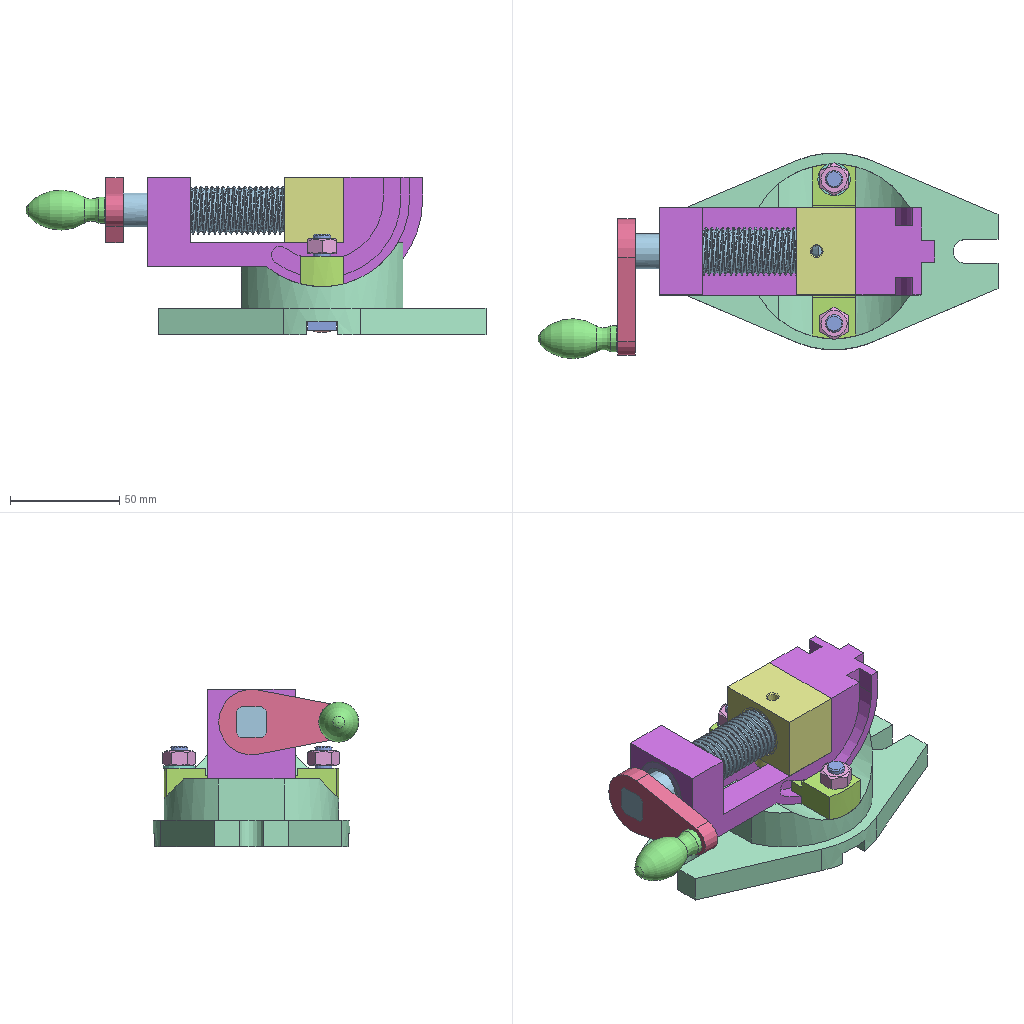Assembly | NX | 12 different items | 15 placed | box 210 x 94 x 72 mm
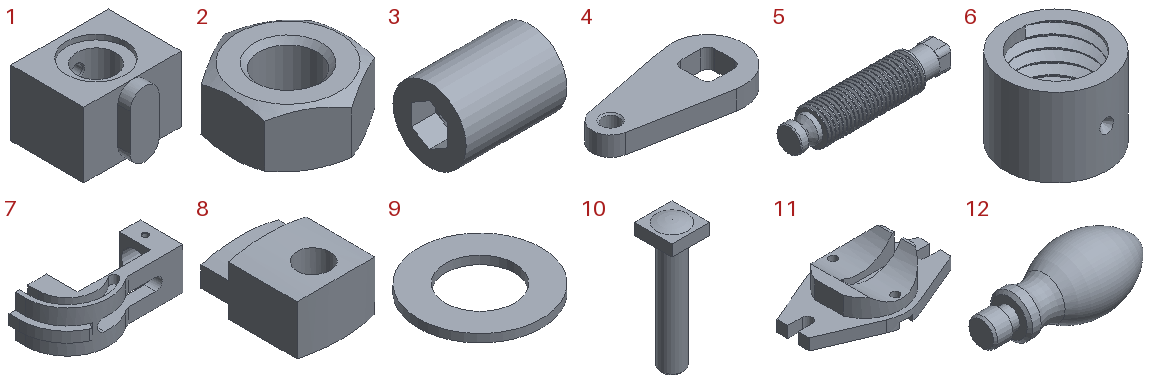Parts list (item | quantity | size | volume | features):
1 | x1 | 40 x 35 x 27 mm | 30203 mm3 | features DATUM_CSYS 6, SKETCH 5, EXTRUDE 4, BLEND 1, HOLE PACKAGE 1, SIMPLE HOLE 1, SYMBOLIC_THREAD 1
2 | x2 | 12.99 x 15 x 6.8 mm | 720.374 mm3 | features DATUM_CSYS 3, EXTRACT_DATUM_AXIS 2, EXTRACT_STRING 2, SKETCH 2, SWP104 2, EXTRUDE 1, HOLE PACKAGE 1, Instance Feature 1, Mirror Feature 1, SIMPLE HOLE 1, SYMBOLIC_THREAD 1
3 | x1 | 10 x 6 x 6 mm | 232.466 mm3 | features DATUM_CSYS 4, SKETCH 3, SWP104 2, EXTRUDE 1
4 | x1 | 62.5 x 30 x 8 mm | 9056 mm3 | features DATUM_CSYS 2, BLEND 1, EXTRUDE 1, HOLE PACKAGE 1, SIMPLE HOLE 1, SKETCH 1, SYMBOLIC_THREAD 1
5 | x1 | 97 x 22 x 22 mm | 27588 mm3 | features DATUM_CSYS 3, SKETCH 2, BLEND 1, CHAMFER 1, EXTRUDE 1, SWP104 1, THREADS 1
6 | x1 | 26 x 26.176 x 20 mm | 3632 mm3 | features DATUM_CSYS 3, SKETCH 2, EXTRUDE 1, SWP104 1, THREADS 1
7 | x1 | 126 x 51.679 x 40 mm | 90129 mm3 | features DATUM_CSYS 8, EXTRUDE 7, SKETCH 7, CPROJ 3, BLEND 2, EXTRACT_FACE 2, EXTRACT_STRING 2, HOLE PACKAGE 1, Instance Feature 1, Mirror Feature 1, SIMPLE HOLE 1, SYMBOLIC_THREAD 1
8 | x2 | 20 x 26 x 14 mm | 4969 mm3 | features DATUM_CSYS 4, EXTRUDE 3, SKETCH 3
9 | x1 | 15 x 15 x 1 mm | 121.297 mm3 | features DATUM_CSYS 2, EXTRUDE 1, SKETCH 1
10 | x2 | 13 x 13 x 45 mm | 2728 mm3 | features DATUM_CSYS 4, SKETCH 3, EXTRUDE 2, CHAMFER 1, SWP104 1
11 | x1 | 150 x 90 x 42 mm | 169157 mm3 | features DATUM_CSYS 6, EXTRUDE 5, SKETCH 5, CPROJ 1, DATUM_PLANE 1
12 | x1 | 44.482 x 18.329 x 18.329 mm | 6113 mm3 | features CHAMFER 2, DATUM_CSYS 2, SKETCH 1, SWP104 1
Mates (type | each side: item.copy, entity, surface, feature):
Fix | 11.1 component
Touch | 7.1 face plane Extrude(9) | 11.1 face plane Extrude(11)
Touch | 7.1 face cylinder Extrude(2) | 11.1 face cylinder Extrude(8)
Touch | 1.1 face plane Extrude(2) | 7.1 face plane Extrude(2)
Touch | 1.1 face plane Extrude(2) | 7.1 face plane Extrude(4) | 2 times
AlignLock | 5.1 face cylinder Threads(3) | 1.1 face cylinder Extrude(9)
Touch | 5.1 face plane Revolve(2) | 1.1 face plane Extrude(9)
AlignLock | 12.1 face cylinder Revolve(2) | 4.1 face cylinder Extrude(2)
Touch | 12.1 edge | 4.1 face plane Extrude(2)
AlignLock | 8.1 face cylinder Extrude(4) | 11.1 face cylinder Extrude(8)
AlignLock | 8.1 face cylinder Extrude(2) | 11.1 face cylinder Extrude(4)
AlignLock | 6.1 face cylinder Extrude(2) | 5.1 face cylinder Revolve(2)
Touch | 6.1 face plane Extrude(2) | 7.1 face plane Extrude(4)
AlignLock | 7.1 face cylinder M6 x 1.0 Threaded Hole(14) | 3.1 face cylinder Revolve(2)
Touch | 3.1 face plane Revolve(2) | 7.1 face plane Extrude(2)
AlignLock | 8.1 face cylinder Extrude(2) | 10.1 face cylinder Extrude(4)
Touch | 10.1 face plane Extrude(2) | 11.1 face plane Extrude(8)
AlignLock | 9.1 face cylinder Extrude(2) | 10.1 face cylinder Extrude(4)
Touch | 9.1 face plane Extrude(2) | 8.1 face plane Extrude(2)
AlignLock | 2.1 face cylinder M8 x 1.25 Threaded Hole(7) | 10.1 face cylinder Extrude(4)
Touch | 2.1 face plane Extrude(2) | 9.1 face plane Extrude(2)
Concentric | 4.1 edge | 5.1 edge
Concentric | 5.1 edge | 4.1 edge